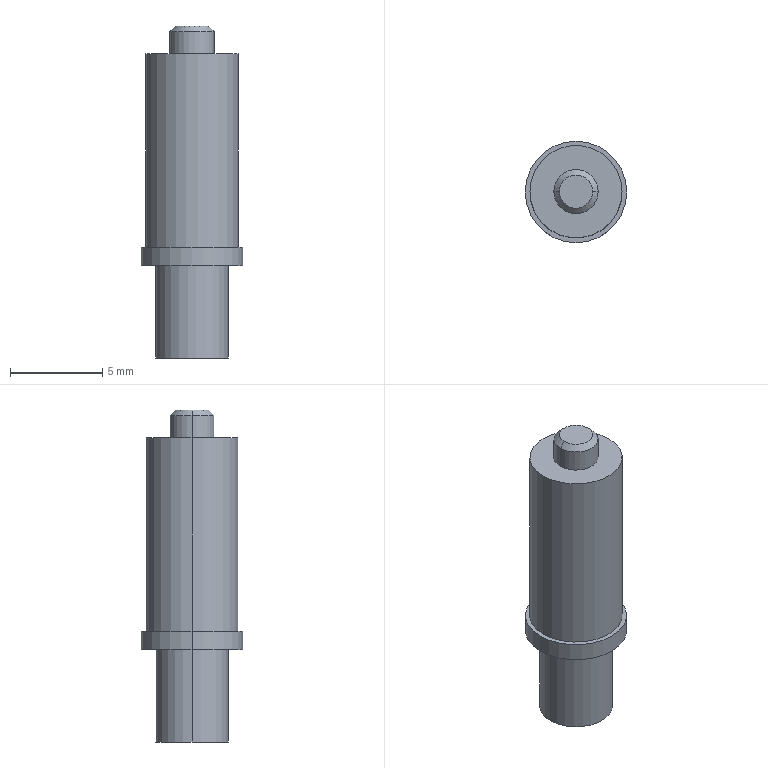Part | STEP file | 1 solid | 21 faces | box 5.5 x 5.5 x 18 mm | volume 266.671 mm3 | cylinder 10 | cone 6 | plane 5 | commonest cylinder face diameters 2.4 x2 2.5 x2 3.95 x2 5 x2 5.5 x2
STEP:
#1=CARTESIAN_POINT('',(0.,0.,0.));
#2=DIRECTION('',(0.,0.,1.));
#3=DIRECTION('',(1.,0.,0.));
#4=AXIS2_PLACEMENT_3D('',#1,#2,#3);
#5=CARTESIAN_POINT('',(-1.25,0.,0.275));
#6=VERTEX_POINT('',#5);
#7=CARTESIAN_POINT('',(-1.525,0.,0.));
#8=VERTEX_POINT('',#7);
#9=CARTESIAN_POINT('',(-1.525,0.,0.));
#10=DIRECTION('',(-0.7071,0.,-0.7071));
#11=VECTOR('',#10,1.);
#12=LINE('',#9,#11);
#13=CARTESIAN_POINT('',(0.,0.,0.));
#14=DIRECTION('',(0.,0.,-1.));
#15=DIRECTION('',(-1.,0.,0.));
#16=AXIS2_PLACEMENT_3D('',#13,#14,#15);
#17=CONICAL_SURFACE('',#16,1.525,0.7854);
#18=CARTESIAN_POINT('',(6.283,0.));
#19=DIRECTION('',(0.,1.));
#20=VECTOR('',#19,1.);
#21=LINE('',#18,#20);
#22=(GEOMETRIC_REPRESENTATION_CONTEXT(2)PARAMETRIC_REPRESENTATION_CONTEXT()REPRESENTATION_CONTEXT('',''));
#23=DEFINITIONAL_REPRESENTATION('',(#21),#22);
#24=PCURVE('',#17,#23);
#25=CARTESIAN_POINT('',(0.,0.,0.));
#26=DIRECTION('',(0.,0.,-1.));
#27=DIRECTION('',(-1.,0.,0.));
#28=AXIS2_PLACEMENT_3D('',#25,#26,#27);
#29=CONICAL_SURFACE('',#28,1.525,0.7854);
#30=CARTESIAN_POINT('',(0.,0.));
#31=DIRECTION('',(0.,1.));
#32=VECTOR('',#31,1.);
#33=LINE('',#30,#32);
#34=(GEOMETRIC_REPRESENTATION_CONTEXT(2)PARAMETRIC_REPRESENTATION_CONTEXT()REPRESENTATION_CONTEXT('',''));
#35=DEFINITIONAL_REPRESENTATION('',(#33),#34);
#36=PCURVE('',#29,#35);
#37=SURFACE_CURVE('',#12,(#24,#36),.PCURVE_S1.);
#38=EDGE_CURVE('',#6,#8,#37,.T.);
#39=ORIENTED_EDGE('',*,*,#38,.T.);
#40=CARTESIAN_POINT('',(1.525,0.,0.));
#41=VERTEX_POINT('',#40);
#42=CARTESIAN_POINT('',(0.,0.,0.));
#43=DIRECTION('',(0.,0.,-1.));
#44=DIRECTION('',(-1.,0.,0.));
#45=AXIS2_PLACEMENT_3D('',#42,#43,#44);
#46=CIRCLE('',#45,1.525);
#47=CARTESIAN_POINT('',(0.,0.));
#48=DIRECTION('',(1.,0.));
#49=VECTOR('',#48,1.);
#50=LINE('',#47,#49);
#51=(GEOMETRIC_REPRESENTATION_CONTEXT(2)PARAMETRIC_REPRESENTATION_CONTEXT()REPRESENTATION_CONTEXT('',''));
#52=DEFINITIONAL_REPRESENTATION('',(#50),#51);
#53=PCURVE('',#17,#52);
#54=CARTESIAN_POINT('',(0.,0.,0.));
#55=DIRECTION('',(0.,0.,-1.));
#56=DIRECTION('',(-1.,0.,0.));
#57=AXIS2_PLACEMENT_3D('',#54,#55,#56);
#58=PLANE('',#57);
#59=CARTESIAN_POINT('',(0.,0.));
#60=DIRECTION('',(1.,0.));
#61=AXIS2_PLACEMENT_2D('',#59,#60);
#62=CIRCLE('',#61,1.525);
#63=(GEOMETRIC_REPRESENTATION_CONTEXT(2)PARAMETRIC_REPRESENTATION_CONTEXT()REPRESENTATION_CONTEXT('',''));
#64=DEFINITIONAL_REPRESENTATION('',(#62),#63);
#65=PCURVE('',#58,#64);
#66=SURFACE_CURVE('',#46,(#53,#65),.PCURVE_S1.);
#67=EDGE_CURVE('',#41,#8,#66,.T.);
#68=ORIENTED_EDGE('',*,*,#67,.F.);
#69=CARTESIAN_POINT('',(1.25,0.,0.275));
#70=VERTEX_POINT('',#69);
#71=CARTESIAN_POINT('',(1.525,0.,0.));
#72=DIRECTION('',(0.7071,0.,-0.7071));
#73=VECTOR('',#72,1.);
#74=LINE('',#71,#73);
#75=CARTESIAN_POINT('',(3.142,0.));
#76=DIRECTION('',(0.,1.));
#77=VECTOR('',#76,1.);
#78=LINE('',#75,#77);
#79=(GEOMETRIC_REPRESENTATION_CONTEXT(2)PARAMETRIC_REPRESENTATION_CONTEXT()REPRESENTATION_CONTEXT('',''));
#80=DEFINITIONAL_REPRESENTATION('',(#78),#79);
#81=PCURVE('',#17,#80);
#82=CARTESIAN_POINT('',(3.142,0.));
#83=DIRECTION('',(0.,1.));
#84=VECTOR('',#83,1.);
#85=LINE('',#82,#84);
#86=(GEOMETRIC_REPRESENTATION_CONTEXT(2)PARAMETRIC_REPRESENTATION_CONTEXT()REPRESENTATION_CONTEXT('',''));
#87=DEFINITIONAL_REPRESENTATION('',(#85),#86);
#88=PCURVE('',#29,#87);
#89=SURFACE_CURVE('',#74,(#81,#88),.PCURVE_S1.);
#90=EDGE_CURVE('',#70,#41,#89,.T.);
#91=ORIENTED_EDGE('',*,*,#90,.F.);
#92=CARTESIAN_POINT('',(0.,0.,0.275));
#93=DIRECTION('',(0.,0.,-1.));
#94=DIRECTION('',(-1.,0.,0.));
#95=AXIS2_PLACEMENT_3D('',#92,#93,#94);
#96=CIRCLE('',#95,1.25);
#97=CARTESIAN_POINT('',(0.,-0.275));
#98=DIRECTION('',(1.,0.));
#99=VECTOR('',#98,1.);
#100=LINE('',#97,#99);
#101=(GEOMETRIC_REPRESENTATION_CONTEXT(2)PARAMETRIC_REPRESENTATION_CONTEXT()REPRESENTATION_CONTEXT('',''));
#102=DEFINITIONAL_REPRESENTATION('',(#100),#101);
#103=PCURVE('',#17,#102);
#104=CARTESIAN_POINT('',(0.,0.,0.));
#105=DIRECTION('',(0.,0.,-1.));
#106=DIRECTION('',(-1.,0.,0.));
#107=AXIS2_PLACEMENT_3D('',#104,#105,#106);
#108=CYLINDRICAL_SURFACE('',#107,1.25);
#109=CARTESIAN_POINT('',(0.,-0.275));
#110=DIRECTION('',(1.,0.));
#111=VECTOR('',#110,1.);
#112=LINE('',#109,#111);
#113=(GEOMETRIC_REPRESENTATION_CONTEXT(2)PARAMETRIC_REPRESENTATION_CONTEXT()REPRESENTATION_CONTEXT('',''));
#114=DEFINITIONAL_REPRESENTATION('',(#112),#113);
#115=PCURVE('',#108,#114);
#116=SURFACE_CURVE('',#96,(#103,#115),.PCURVE_S1.);
#117=EDGE_CURVE('',#70,#6,#116,.T.);
#118=ORIENTED_EDGE('',*,*,#117,.T.);
#119=EDGE_LOOP('',(#39,#68,#91,#118));
#120=FACE_BOUND('',#119,.F.);
#121=ADVANCED_FACE('',(#120),#17,.F.);
#122=CARTESIAN_POINT('',(-1.25,0.,6.));
#123=VERTEX_POINT('',#122);
#124=CARTESIAN_POINT('',(-1.25,0.,0.));
#125=DIRECTION('',(0.,0.,-1.));
#126=VECTOR('',#125,1.);
#127=LINE('',#124,#126);
#128=CARTESIAN_POINT('',(6.283,0.));
#129=DIRECTION('',(0.,1.));
#130=VECTOR('',#129,1.);
#131=LINE('',#128,#130);
#132=(GEOMETRIC_REPRESENTATION_CONTEXT(2)PARAMETRIC_REPRESENTATION_CONTEXT()REPRESENTATION_CONTEXT('',''));
#133=DEFINITIONAL_REPRESENTATION('',(#131),#132);
#134=PCURVE('',#108,#133);
#135=CARTESIAN_POINT('',(0.,0.,0.));
#136=DIRECTION('',(0.,0.,-1.));
#137=DIRECTION('',(-1.,0.,0.));
#138=AXIS2_PLACEMENT_3D('',#135,#136,#137);
#139=CYLINDRICAL_SURFACE('',#138,1.25);
#140=CARTESIAN_POINT('',(0.,0.));
#141=DIRECTION('',(0.,1.));
#142=VECTOR('',#141,1.);
#143=LINE('',#140,#142);
#144=(GEOMETRIC_REPRESENTATION_CONTEXT(2)PARAMETRIC_REPRESENTATION_CONTEXT()REPRESENTATION_CONTEXT('',''));
#145=DEFINITIONAL_REPRESENTATION('',(#143),#144);
#146=PCURVE('',#139,#145);
#147=SURFACE_CURVE('',#127,(#134,#146),.PCURVE_S1.);
#148=EDGE_CURVE('',#123,#6,#147,.T.);
#149=ORIENTED_EDGE('',*,*,#148,.T.);
#150=ORIENTED_EDGE('',*,*,#117,.F.);
#151=CARTESIAN_POINT('',(1.25,0.,6.));
#152=VERTEX_POINT('',#151);
#153=CARTESIAN_POINT('',(1.25,0.,0.));
#154=DIRECTION('',(0.,0.,-1.));
#155=VECTOR('',#154,1.);
#156=LINE('',#153,#155);
#157=CARTESIAN_POINT('',(3.142,0.));
#158=DIRECTION('',(0.,1.));
#159=VECTOR('',#158,1.);
#160=LINE('',#157,#159);
#161=(GEOMETRIC_REPRESENTATION_CONTEXT(2)PARAMETRIC_REPRESENTATION_CONTEXT()REPRESENTATION_CONTEXT('',''));
#162=DEFINITIONAL_REPRESENTATION('',(#160),#161);
#163=PCURVE('',#108,#162);
#164=CARTESIAN_POINT('',(3.142,0.));
#165=DIRECTION('',(0.,1.));
#166=VECTOR('',#165,1.);
#167=LINE('',#164,#166);
#168=(GEOMETRIC_REPRESENTATION_CONTEXT(2)PARAMETRIC_REPRESENTATION_CONTEXT()REPRESENTATION_CONTEXT('',''));
#169=DEFINITIONAL_REPRESENTATION('',(#167),#168);
#170=PCURVE('',#139,#169);
#171=SURFACE_CURVE('',#156,(#163,#170),.PCURVE_S1.);
#172=EDGE_CURVE('',#152,#70,#171,.T.);
#173=ORIENTED_EDGE('',*,*,#172,.F.);
#174=CARTESIAN_POINT('',(0.,0.,6.));
#175=DIRECTION('',(0.,0.,-1.));
#176=DIRECTION('',(-1.,0.,0.));
#177=AXIS2_PLACEMENT_3D('',#174,#175,#176);
#178=CIRCLE('',#177,1.25);
#179=CARTESIAN_POINT('',(0.,-6.));
#180=DIRECTION('',(1.,0.));
#181=VECTOR('',#180,1.);
#182=LINE('',#179,#181);
#183=(GEOMETRIC_REPRESENTATION_CONTEXT(2)PARAMETRIC_REPRESENTATION_CONTEXT()REPRESENTATION_CONTEXT('',''));
#184=DEFINITIONAL_REPRESENTATION('',(#182),#183);
#185=PCURVE('',#108,#184);
#186=CARTESIAN_POINT('',(0.,0.,6.));
#187=DIRECTION('',(0.,0.,-1.));
#188=DIRECTION('',(-1.,0.,0.));
#189=AXIS2_PLACEMENT_3D('',#186,#187,#188);
#190=CONICAL_SURFACE('',#189,1.25,1.03);
#191=CARTESIAN_POINT('',(0.,0.));
#192=DIRECTION('',(1.,0.));
#193=VECTOR('',#192,1.);
#194=LINE('',#191,#193);
#195=(GEOMETRIC_REPRESENTATION_CONTEXT(2)PARAMETRIC_REPRESENTATION_CONTEXT()REPRESENTATION_CONTEXT('',''));
#196=DEFINITIONAL_REPRESENTATION('',(#194),#195);
#197=PCURVE('',#190,#196);
#198=SURFACE_CURVE('',#178,(#185,#197),.PCURVE_S1.);
#199=EDGE_CURVE('',#152,#123,#198,.T.);
#200=ORIENTED_EDGE('',*,*,#199,.T.);
#201=EDGE_LOOP('',(#149,#150,#173,#200));
#202=FACE_BOUND('',#201,.F.);
#203=ADVANCED_FACE('',(#202),#108,.F.);
#204=ORIENTED_EDGE('',*,*,#199,.F.);
#205=CARTESIAN_POINT('',(0.,0.,6.751));
#206=VERTEX_POINT('',#205);
#207=CARTESIAN_POINT('',(1.25,0.,6.));
#208=DIRECTION('',(0.8572,0.,-0.515));
#209=VECTOR('',#208,1.);
#210=LINE('',#207,#209);
#211=CARTESIAN_POINT('',(3.142,0.));
#212=DIRECTION('',(0.,1.));
#213=VECTOR('',#212,1.);
#214=LINE('',#211,#213);
#215=(GEOMETRIC_REPRESENTATION_CONTEXT(2)PARAMETRIC_REPRESENTATION_CONTEXT()REPRESENTATION_CONTEXT('',''));
#216=DEFINITIONAL_REPRESENTATION('',(#214),#215);
#217=PCURVE('',#190,#216);
#218=CARTESIAN_POINT('',(0.,0.,6.));
#219=DIRECTION('',(0.,0.,-1.));
#220=DIRECTION('',(-1.,0.,0.));
#221=AXIS2_PLACEMENT_3D('',#218,#219,#220);
#222=CONICAL_SURFACE('',#221,1.25,1.03);
#223=CARTESIAN_POINT('',(3.142,0.));
#224=DIRECTION('',(0.,1.));
#225=VECTOR('',#224,1.);
#226=LINE('',#223,#225);
#227=(GEOMETRIC_REPRESENTATION_CONTEXT(2)PARAMETRIC_REPRESENTATION_CONTEXT()REPRESENTATION_CONTEXT('',''));
#228=DEFINITIONAL_REPRESENTATION('',(#226),#227);
#229=PCURVE('',#222,#228);
#230=SURFACE_CURVE('',#210,(#217,#229),.PCURVE_S1.);
#231=EDGE_CURVE('',#206,#152,#230,.T.);
#232=ORIENTED_EDGE('',*,*,#231,.F.);
#233=CARTESIAN_POINT('',(-1.25,0.,6.));
#234=DIRECTION('',(-0.8572,0.,-0.515));
#235=VECTOR('',#234,1.);
#236=LINE('',#233,#235);
#237=CARTESIAN_POINT('',(6.283,0.));
#238=DIRECTION('',(0.,1.));
#239=VECTOR('',#238,1.);
#240=LINE('',#237,#239);
#241=(GEOMETRIC_REPRESENTATION_CONTEXT(2)PARAMETRIC_REPRESENTATION_CONTEXT()REPRESENTATION_CONTEXT('',''));
#242=DEFINITIONAL_REPRESENTATION('',(#240),#241);
#243=PCURVE('',#190,#242);
#244=CARTESIAN_POINT('',(0.,0.));
#245=DIRECTION('',(0.,1.));
#246=VECTOR('',#245,1.);
#247=LINE('',#244,#246);
#248=(GEOMETRIC_REPRESENTATION_CONTEXT(2)PARAMETRIC_REPRESENTATION_CONTEXT()REPRESENTATION_CONTEXT('',''));
#249=DEFINITIONAL_REPRESENTATION('',(#247),#248);
#250=PCURVE('',#222,#249);
#251=SURFACE_CURVE('',#236,(#243,#250),.PCURVE_S1.);
#252=EDGE_CURVE('',#206,#123,#251,.T.);
#253=ORIENTED_EDGE('',*,*,#252,.T.);
#254=EDGE_LOOP('',(#204,#232,#253));
#255=FACE_BOUND('',#254,.F.);
#256=ADVANCED_FACE('',(#255),#190,.F.);
#257=CARTESIAN_POINT('',(0.9,0.,18.));
#258=VERTEX_POINT('',#257);
#259=CARTESIAN_POINT('',(-0.9,0.,18.));
#260=VERTEX_POINT('',#259);
#261=CARTESIAN_POINT('',(0.,0.,18.));
#262=DIRECTION('',(0.,0.,1.));
#263=DIRECTION('',(1.,0.,0.));
#264=AXIS2_PLACEMENT_3D('',#261,#262,#263);
#265=CIRCLE('',#264,0.9);
#266=CARTESIAN_POINT('',(0.,0.,18.));
#267=DIRECTION('',(0.,0.,-1.));
#268=DIRECTION('',(-1.,0.,0.));
#269=AXIS2_PLACEMENT_3D('',#266,#267,#268);
#270=CONICAL_SURFACE('',#269,0.9,0.7854);
#271=CARTESIAN_POINT('',(3.142,0.));
#272=DIRECTION('',(-1.,0.));
#273=VECTOR('',#272,1.);
#274=LINE('',#271,#273);
#275=(GEOMETRIC_REPRESENTATION_CONTEXT(2)PARAMETRIC_REPRESENTATION_CONTEXT()REPRESENTATION_CONTEXT('',''));
#276=DEFINITIONAL_REPRESENTATION('',(#274),#275);
#277=PCURVE('',#270,#276);
#278=CARTESIAN_POINT('',(0.9,0.,18.));
#279=DIRECTION('',(0.,0.,1.));
#280=DIRECTION('',(1.,0.,0.));
#281=AXIS2_PLACEMENT_3D('',#278,#279,#280);
#282=PLANE('',#281);
#283=CARTESIAN_POINT('',(-0.9,0.));
#284=DIRECTION('',(1.,0.));
#285=AXIS2_PLACEMENT_2D('',#283,#284);
#286=CIRCLE('',#285,0.9);
#287=(GEOMETRIC_REPRESENTATION_CONTEXT(2)PARAMETRIC_REPRESENTATION_CONTEXT()REPRESENTATION_CONTEXT('',''));
#288=DEFINITIONAL_REPRESENTATION('',(#286),#287);
#289=PCURVE('',#282,#288);
#290=SURFACE_CURVE('',#265,(#277,#289),.PCURVE_S1.);
#291=EDGE_CURVE('',#258,#260,#290,.T.);
#292=ORIENTED_EDGE('',*,*,#291,.F.);
#293=CARTESIAN_POINT('',(1.2,0.,17.7));
#294=VERTEX_POINT('',#293);
#295=CARTESIAN_POINT('',(0.9,0.,18.));
#296=DIRECTION('',(0.7071,0.,-0.7071));
#297=VECTOR('',#296,1.);
#298=LINE('',#295,#297);
#299=CARTESIAN_POINT('',(3.142,0.));
#300=DIRECTION('',(0.,1.));
#301=VECTOR('',#300,1.);
#302=LINE('',#299,#301);
#303=(GEOMETRIC_REPRESENTATION_CONTEXT(2)PARAMETRIC_REPRESENTATION_CONTEXT()REPRESENTATION_CONTEXT('',''));
#304=DEFINITIONAL_REPRESENTATION('',(#302),#303);
#305=PCURVE('',#270,#304);
#306=CARTESIAN_POINT('',(0.,0.,18.));
#307=DIRECTION('',(0.,0.,-1.));
#308=DIRECTION('',(-1.,0.,0.));
#309=AXIS2_PLACEMENT_3D('',#306,#307,#308);
#310=CONICAL_SURFACE('',#309,0.9,0.7854);
#311=CARTESIAN_POINT('',(3.142,0.));
#312=DIRECTION('',(0.,1.));
#313=VECTOR('',#312,1.);
#314=LINE('',#311,#313);
#315=(GEOMETRIC_REPRESENTATION_CONTEXT(2)PARAMETRIC_REPRESENTATION_CONTEXT()REPRESENTATION_CONTEXT('',''));
#316=DEFINITIONAL_REPRESENTATION('',(#314),#315);
#317=PCURVE('',#310,#316);
#318=SURFACE_CURVE('',#298,(#305,#317),.PCURVE_S1.);
#319=EDGE_CURVE('',#258,#294,#318,.T.);
#320=ORIENTED_EDGE('',*,*,#319,.T.);
#321=CARTESIAN_POINT('',(-1.2,0.,17.7));
#322=VERTEX_POINT('',#321);
#323=CARTESIAN_POINT('',(0.,0.,17.7));
#324=DIRECTION('',(0.,0.,1.));
#325=DIRECTION('',(1.,0.,0.));
#326=AXIS2_PLACEMENT_3D('',#323,#324,#325);
#327=CIRCLE('',#326,1.2);
#328=CARTESIAN_POINT('',(3.142,0.3));
#329=DIRECTION('',(-1.,0.));
#330=VECTOR('',#329,1.);
#331=LINE('',#328,#330);
#332=(GEOMETRIC_REPRESENTATION_CONTEXT(2)PARAMETRIC_REPRESENTATION_CONTEXT()REPRESENTATION_CONTEXT('',''));
#333=DEFINITIONAL_REPRESENTATION('',(#331),#332);
#334=PCURVE('',#270,#333);
#335=CARTESIAN_POINT('',(0.,0.,0.));
#336=DIRECTION('',(0.,0.,1.));
#337=DIRECTION('',(1.,0.,0.));
#338=AXIS2_PLACEMENT_3D('',#335,#336,#337);
#339=CYLINDRICAL_SURFACE('',#338,1.2);
#340=CARTESIAN_POINT('',(0.,17.7));
#341=DIRECTION('',(1.,0.));
#342=VECTOR('',#341,1.);
#343=LINE('',#340,#342);
#344=(GEOMETRIC_REPRESENTATION_CONTEXT(2)PARAMETRIC_REPRESENTATION_CONTEXT()REPRESENTATION_CONTEXT('',''));
#345=DEFINITIONAL_REPRESENTATION('',(#343),#344);
#346=PCURVE('',#339,#345);
#347=SURFACE_CURVE('',#327,(#334,#346),.PCURVE_S1.);
#348=EDGE_CURVE('',#294,#322,#347,.T.);
#349=ORIENTED_EDGE('',*,*,#348,.T.);
#350=CARTESIAN_POINT('',(-0.9,0.,18.));
#351=DIRECTION('',(-0.7071,0.,-0.7071));
#352=VECTOR('',#351,1.);
#353=LINE('',#350,#352);
#354=CARTESIAN_POINT('',(0.,0.));
#355=DIRECTION('',(0.,1.));
#356=VECTOR('',#355,1.);
#357=LINE('',#354,#356);
#358=(GEOMETRIC_REPRESENTATION_CONTEXT(2)PARAMETRIC_REPRESENTATION_CONTEXT()REPRESENTATION_CONTEXT('',''));
#359=DEFINITIONAL_REPRESENTATION('',(#357),#358);
#360=PCURVE('',#270,#359);
#361=CARTESIAN_POINT('',(6.283,0.));
#362=DIRECTION('',(0.,1.));
#363=VECTOR('',#362,1.);
#364=LINE('',#361,#363);
#365=(GEOMETRIC_REPRESENTATION_CONTEXT(2)PARAMETRIC_REPRESENTATION_CONTEXT()REPRESENTATION_CONTEXT('',''));
#366=DEFINITIONAL_REPRESENTATION('',(#364),#365);
#367=PCURVE('',#310,#366);
#368=SURFACE_CURVE('',#353,(#360,#367),.PCURVE_S1.);
#369=EDGE_CURVE('',#260,#322,#368,.T.);
#370=ORIENTED_EDGE('',*,*,#369,.F.);
#371=EDGE_LOOP('',(#292,#320,#349,#370));
#372=FACE_BOUND('',#371,.T.);
#373=ADVANCED_FACE('',(#372),#270,.T.);
#374=CARTESIAN_POINT('',(1.2,0.,16.5));
#375=VERTEX_POINT('',#374);
#376=CARTESIAN_POINT('',(-1.2,0.,16.5));
#377=VERTEX_POINT('',#376);
#378=CARTESIAN_POINT('',(0.,0.,16.5));
#379=DIRECTION('',(0.,0.,1.));
#380=DIRECTION('',(1.,0.,0.));
#381=AXIS2_PLACEMENT_3D('',#378,#379,#380);
#382=CIRCLE('',#381,1.2);
#383=CARTESIAN_POINT('',(0.,16.5));
#384=DIRECTION('',(1.,0.));
#385=VECTOR('',#384,1.);
#386=LINE('',#383,#385);
#387=(GEOMETRIC_REPRESENTATION_CONTEXT(2)PARAMETRIC_REPRESENTATION_CONTEXT()REPRESENTATION_CONTEXT('',''));
#388=DEFINITIONAL_REPRESENTATION('',(#386),#387);
#389=PCURVE('',#339,#388);
#390=CARTESIAN_POINT('',(2.5,0.,16.5));
#391=DIRECTION('',(0.,0.,1.));
#392=DIRECTION('',(1.,0.,0.));
#393=AXIS2_PLACEMENT_3D('',#390,#391,#392);
#394=PLANE('',#393);
#395=CARTESIAN_POINT('',(-2.5,0.));
#396=DIRECTION('',(1.,0.));
#397=AXIS2_PLACEMENT_2D('',#395,#396);
#398=CIRCLE('',#397,1.2);
#399=(GEOMETRIC_REPRESENTATION_CONTEXT(2)PARAMETRIC_REPRESENTATION_CONTEXT()REPRESENTATION_CONTEXT('',''));
#400=DEFINITIONAL_REPRESENTATION('',(#398),#399);
#401=PCURVE('',#394,#400);
#402=SURFACE_CURVE('',#382,(#389,#401),.PCURVE_S1.);
#403=EDGE_CURVE('',#375,#377,#402,.T.);
#404=ORIENTED_EDGE('',*,*,#403,.T.);
#405=CARTESIAN_POINT('',(-1.2,0.,0.));
#406=DIRECTION('',(0.,0.,1.));
#407=VECTOR('',#406,1.);
#408=LINE('',#405,#407);
#409=CARTESIAN_POINT('',(3.142,0.));
#410=DIRECTION('',(0.,1.));
#411=VECTOR('',#410,1.);
#412=LINE('',#409,#411);
#413=(GEOMETRIC_REPRESENTATION_CONTEXT(2)PARAMETRIC_REPRESENTATION_CONTEXT()REPRESENTATION_CONTEXT('',''));
#414=DEFINITIONAL_REPRESENTATION('',(#412),#413);
#415=PCURVE('',#339,#414);
#416=CARTESIAN_POINT('',(0.,0.,0.));
#417=DIRECTION('',(0.,0.,1.));
#418=DIRECTION('',(1.,0.,0.));
#419=AXIS2_PLACEMENT_3D('',#416,#417,#418);
#420=CYLINDRICAL_SURFACE('',#419,1.2);
#421=CARTESIAN_POINT('',(3.142,0.));
#422=DIRECTION('',(0.,1.));
#423=VECTOR('',#422,1.);
#424=LINE('',#421,#423);
#425=(GEOMETRIC_REPRESENTATION_CONTEXT(2)PARAMETRIC_REPRESENTATION_CONTEXT()REPRESENTATION_CONTEXT('',''));
#426=DEFINITIONAL_REPRESENTATION('',(#424),#425);
#427=PCURVE('',#420,#426);
#428=SURFACE_CURVE('',#408,(#415,#427),.PCURVE_S1.);
#429=EDGE_CURVE('',#377,#322,#428,.T.);
#430=ORIENTED_EDGE('',*,*,#429,.T.);
#431=ORIENTED_EDGE('',*,*,#348,.F.);
#432=CARTESIAN_POINT('',(1.2,0.,0.));
#433=DIRECTION('',(0.,0.,1.));
#434=VECTOR('',#433,1.);
#435=LINE('',#432,#434);
#436=CARTESIAN_POINT('',(0.,0.));
#437=DIRECTION('',(0.,1.));
#438=VECTOR('',#437,1.);
#439=LINE('',#436,#438);
#440=(GEOMETRIC_REPRESENTATION_CONTEXT(2)PARAMETRIC_REPRESENTATION_CONTEXT()REPRESENTATION_CONTEXT('',''));
#441=DEFINITIONAL_REPRESENTATION('',(#439),#440);
#442=PCURVE('',#339,#441);
#443=CARTESIAN_POINT('',(6.283,0.));
#444=DIRECTION('',(0.,1.));
#445=VECTOR('',#444,1.);
#446=LINE('',#443,#445);
#447=(GEOMETRIC_REPRESENTATION_CONTEXT(2)PARAMETRIC_REPRESENTATION_CONTEXT()REPRESENTATION_CONTEXT('',''));
#448=DEFINITIONAL_REPRESENTATION('',(#446),#447);
#449=PCURVE('',#420,#448);
#450=SURFACE_CURVE('',#435,(#442,#449),.PCURVE_S1.);
#451=EDGE_CURVE('',#375,#294,#450,.T.);
#452=ORIENTED_EDGE('',*,*,#451,.F.);
#453=EDGE_LOOP('',(#404,#430,#431,#452));
#454=FACE_BOUND('',#453,.T.);
#455=ADVANCED_FACE('',(#454),#339,.T.);
#456=CARTESIAN_POINT('',(2.5,0.,6.));
#457=VERTEX_POINT('',#456);
#458=CARTESIAN_POINT('',(-2.5,0.,6.));
#459=VERTEX_POINT('',#458);
#460=CARTESIAN_POINT('',(0.,0.,6.));
#461=DIRECTION('',(0.,0.,1.));
#462=DIRECTION('',(1.,0.,0.));
#463=AXIS2_PLACEMENT_3D('',#460,#461,#462);
#464=CIRCLE('',#463,2.5);
#465=CARTESIAN_POINT('',(0.,0.,0.));
#466=DIRECTION('',(0.,0.,1.));
#467=DIRECTION('',(1.,0.,0.));
#468=AXIS2_PLACEMENT_3D('',#465,#466,#467);
#469=CYLINDRICAL_SURFACE('',#468,2.5);
#470=CARTESIAN_POINT('',(0.,6.));
#471=DIRECTION('',(1.,0.));
#472=VECTOR('',#471,1.);
#473=LINE('',#470,#472);
#474=(GEOMETRIC_REPRESENTATION_CONTEXT(2)PARAMETRIC_REPRESENTATION_CONTEXT()REPRESENTATION_CONTEXT('',''));
#475=DEFINITIONAL_REPRESENTATION('',(#473),#474);
#476=PCURVE('',#469,#475);
#477=CARTESIAN_POINT('',(2.75,0.,6.));
#478=DIRECTION('',(0.,0.,1.));
#479=DIRECTION('',(1.,0.,0.));
#480=AXIS2_PLACEMENT_3D('',#477,#478,#479);
#481=PLANE('',#480);
#482=CARTESIAN_POINT('',(-2.75,0.));
#483=DIRECTION('',(1.,0.));
#484=AXIS2_PLACEMENT_2D('',#482,#483);
#485=CIRCLE('',#484,2.5);
#486=(GEOMETRIC_REPRESENTATION_CONTEXT(2)PARAMETRIC_REPRESENTATION_CONTEXT()REPRESENTATION_CONTEXT('',''));
#487=DEFINITIONAL_REPRESENTATION('',(#485),#486);
#488=PCURVE('',#481,#487);
#489=SURFACE_CURVE('',#464,(#476,#488),.PCURVE_S1.);
#490=EDGE_CURVE('',#457,#459,#489,.T.);
#491=ORIENTED_EDGE('',*,*,#490,.T.);
#492=CARTESIAN_POINT('',(-2.5,0.,16.5));
#493=VERTEX_POINT('',#492);
#494=CARTESIAN_POINT('',(-2.5,0.,0.));
#495=DIRECTION('',(0.,0.,1.));
#496=VECTOR('',#495,1.);
#497=LINE('',#494,#496);
#498=CARTESIAN_POINT('',(3.142,0.));
#499=DIRECTION('',(0.,1.));
#500=VECTOR('',#499,1.);
#501=LINE('',#498,#500);
#502=(GEOMETRIC_REPRESENTATION_CONTEXT(2)PARAMETRIC_REPRESENTATION_CONTEXT()REPRESENTATION_CONTEXT('',''));
#503=DEFINITIONAL_REPRESENTATION('',(#501),#502);
#504=PCURVE('',#469,#503);
#505=CARTESIAN_POINT('',(0.,0.,0.));
#506=DIRECTION('',(0.,0.,1.));
#507=DIRECTION('',(1.,0.,0.));
#508=AXIS2_PLACEMENT_3D('',#505,#506,#507);
#509=CYLINDRICAL_SURFACE('',#508,2.5);
#510=CARTESIAN_POINT('',(3.142,0.));
#511=DIRECTION('',(0.,1.));
#512=VECTOR('',#511,1.);
#513=LINE('',#510,#512);
#514=(GEOMETRIC_REPRESENTATION_CONTEXT(2)PARAMETRIC_REPRESENTATION_CONTEXT()REPRESENTATION_CONTEXT('',''));
#515=DEFINITIONAL_REPRESENTATION('',(#513),#514);
#516=PCURVE('',#509,#515);
#517=SURFACE_CURVE('',#497,(#504,#516),.PCURVE_S1.);
#518=EDGE_CURVE('',#459,#493,#517,.T.);
#519=ORIENTED_EDGE('',*,*,#518,.T.);
#520=CARTESIAN_POINT('',(2.5,0.,16.5));
#521=VERTEX_POINT('',#520);
#522=CARTESIAN_POINT('',(0.,0.,16.5));
#523=DIRECTION('',(0.,0.,1.));
#524=DIRECTION('',(1.,0.,0.));
#525=AXIS2_PLACEMENT_3D('',#522,#523,#524);
#526=CIRCLE('',#525,2.5);
#527=CARTESIAN_POINT('',(0.,16.5));
#528=DIRECTION('',(1.,0.));
#529=VECTOR('',#528,1.);
#530=LINE('',#527,#529);
#531=(GEOMETRIC_REPRESENTATION_CONTEXT(2)PARAMETRIC_REPRESENTATION_CONTEXT()REPRESENTATION_CONTEXT('',''));
#532=DEFINITIONAL_REPRESENTATION('',(#530),#531);
#533=PCURVE('',#469,#532);
#534=CARTESIAN_POINT('',(-2.5,0.));
#535=DIRECTION('',(1.,0.));
#536=AXIS2_PLACEMENT_2D('',#534,#535);
#537=CIRCLE('',#536,2.5);
#538=(GEOMETRIC_REPRESENTATION_CONTEXT(2)PARAMETRIC_REPRESENTATION_CONTEXT()REPRESENTATION_CONTEXT('',''));
#539=DEFINITIONAL_REPRESENTATION('',(#537),#538);
#540=PCURVE('',#394,#539);
#541=SURFACE_CURVE('',#526,(#533,#540),.PCURVE_S1.);
#542=EDGE_CURVE('',#521,#493,#541,.T.);
#543=ORIENTED_EDGE('',*,*,#542,.F.);
#544=CARTESIAN_POINT('',(2.5,0.,0.));
#545=DIRECTION('',(0.,0.,1.));
#546=VECTOR('',#545,1.);
#547=LINE('',#544,#546);
#548=CARTESIAN_POINT('',(0.,0.));
#549=DIRECTION('',(0.,1.));
#550=VECTOR('',#549,1.);
#551=LINE('',#548,#550);
#552=(GEOMETRIC_REPRESENTATION_CONTEXT(2)PARAMETRIC_REPRESENTATION_CONTEXT()REPRESENTATION_CONTEXT('',''));
#553=DEFINITIONAL_REPRESENTATION('',(#551),#552);
#554=PCURVE('',#469,#553);
#555=CARTESIAN_POINT('',(6.283,0.));
#556=DIRECTION('',(0.,1.));
#557=VECTOR('',#556,1.);
#558=LINE('',#555,#557);
#559=(GEOMETRIC_REPRESENTATION_CONTEXT(2)PARAMETRIC_REPRESENTATION_CONTEXT()REPRESENTATION_CONTEXT('',''));
#560=DEFINITIONAL_REPRESENTATION('',(#558),#559);
#561=PCURVE('',#509,#560);
#562=SURFACE_CURVE('',#547,(#554,#561),.PCURVE_S1.);
#563=EDGE_CURVE('',#457,#521,#562,.T.);
#564=ORIENTED_EDGE('',*,*,#563,.F.);
#565=EDGE_LOOP('',(#491,#519,#543,#564));
#566=FACE_BOUND('',#565,.T.);
#567=ADVANCED_FACE('',(#566),#469,.T.);
#568=CARTESIAN_POINT('',(2.75,0.,5.));
#569=VERTEX_POINT('',#568);
#570=CARTESIAN_POINT('',(-2.75,0.,5.));
#571=VERTEX_POINT('',#570);
#572=CARTESIAN_POINT('',(0.,0.,5.));
#573=DIRECTION('',(0.,0.,1.));
#574=DIRECTION('',(1.,0.,0.));
#575=AXIS2_PLACEMENT_3D('',#572,#573,#574);
#576=CIRCLE('',#575,2.75);
#577=CARTESIAN_POINT('',(0.,0.,0.));
#578=DIRECTION('',(0.,0.,1.));
#579=DIRECTION('',(1.,0.,0.));
#580=AXIS2_PLACEMENT_3D('',#577,#578,#579);
#581=CYLINDRICAL_SURFACE('',#580,2.75);
#582=CARTESIAN_POINT('',(0.,5.));
#583=DIRECTION('',(1.,0.));
#584=VECTOR('',#583,1.);
#585=LINE('',#582,#584);
#586=(GEOMETRIC_REPRESENTATION_CONTEXT(2)PARAMETRIC_REPRESENTATION_CONTEXT()REPRESENTATION_CONTEXT('',''));
#587=DEFINITIONAL_REPRESENTATION('',(#585),#586);
#588=PCURVE('',#581,#587);
#589=CARTESIAN_POINT('',(1.975,0.,5.));
#590=DIRECTION('',(0.,0.,-1.));
#591=DIRECTION('',(-1.,0.,0.));
#592=AXIS2_PLACEMENT_3D('',#589,#590,#591);
#593=PLANE('',#592);
#594=CARTESIAN_POINT('',(-0.775,0.));
#595=CARTESIAN_POINT('',(-0.775,4.763));
#596=CARTESIAN_POINT('',(3.35,2.382));
#597=CARTESIAN_POINT('',(7.475,0.));
#598=CARTESIAN_POINT('',(3.35,-2.382));
#599=CARTESIAN_POINT('',(-0.775,-4.763));
#600=CARTESIAN_POINT('',(-0.775,0.));
#601=(BOUNDED_CURVE()B_SPLINE_CURVE(2,(#594,#595,#596,#597,#598,#599,#600),.UNSPECIFIED.,.T.,.F.)B_SPLINE_CURVE_WITH_KNOTS((1,2,2,2,2,1),(-2.094,0.,2.094,4.189,6.283,8.378),.UNSPECIFIED.)CURVE()GEOMETRIC_REPRESENTATION_ITEM()RATIONAL_B_SPLINE_CURVE((1.,0.5,1.,0.5,1.,0.5,1.))REPRESENTATION_ITEM(''));
#602=(GEOMETRIC_REPRESENTATION_CONTEXT(2)PARAMETRIC_REPRESENTATION_CONTEXT()REPRESENTATION_CONTEXT('',''));
#603=DEFINITIONAL_REPRESENTATION('',(#601),#602);
#604=PCURVE('',#593,#603);
#605=SURFACE_CURVE('',#576,(#588,#604),.PCURVE_S1.);
#606=EDGE_CURVE('',#569,#571,#605,.T.);
#607=ORIENTED_EDGE('',*,*,#606,.T.);
#608=CARTESIAN_POINT('',(-2.75,0.,6.));
#609=VERTEX_POINT('',#608);
#610=CARTESIAN_POINT('',(-2.75,0.,0.));
#611=DIRECTION('',(0.,0.,1.));
#612=VECTOR('',#611,1.);
#613=LINE('',#610,#612);
#614=CARTESIAN_POINT('',(3.142,0.));
#615=DIRECTION('',(0.,1.));
#616=VECTOR('',#615,1.);
#617=LINE('',#614,#616);
#618=(GEOMETRIC_REPRESENTATION_CONTEXT(2)PARAMETRIC_REPRESENTATION_CONTEXT()REPRESENTATION_CONTEXT('',''));
#619=DEFINITIONAL_REPRESENTATION('',(#617),#618);
#620=PCURVE('',#581,#619);
#621=CARTESIAN_POINT('',(0.,0.,0.));
#622=DIRECTION('',(0.,0.,1.));
#623=DIRECTION('',(1.,0.,0.));
#624=AXIS2_PLACEMENT_3D('',#621,#622,#623);
#625=CYLINDRICAL_SURFACE('',#624,2.75);
#626=CARTESIAN_POINT('',(3.142,0.));
#627=DIRECTION('',(0.,1.));
#628=VECTOR('',#627,1.);
#629=LINE('',#626,#628);
#630=(GEOMETRIC_REPRESENTATION_CONTEXT(2)PARAMETRIC_REPRESENTATION_CONTEXT()REPRESENTATION_CONTEXT('',''));
#631=DEFINITIONAL_REPRESENTATION('',(#629),#630);
#632=PCURVE('',#625,#631);
#633=SURFACE_CURVE('',#613,(#620,#632),.PCURVE_S1.);
#634=EDGE_CURVE('',#571,#609,#633,.T.);
#635=ORIENTED_EDGE('',*,*,#634,.T.);
#636=CARTESIAN_POINT('',(2.75,0.,6.));
#637=VERTEX_POINT('',#636);
#638=CARTESIAN_POINT('',(0.,0.,6.));
#639=DIRECTION('',(0.,0.,1.));
#640=DIRECTION('',(1.,0.,0.));
#641=AXIS2_PLACEMENT_3D('',#638,#639,#640);
#642=CIRCLE('',#641,2.75);
#643=CARTESIAN_POINT('',(0.,6.));
#644=DIRECTION('',(1.,0.));
#645=VECTOR('',#644,1.);
#646=LINE('',#643,#645);
#647=(GEOMETRIC_REPRESENTATION_CONTEXT(2)PARAMETRIC_REPRESENTATION_CONTEXT()REPRESENTATION_CONTEXT('',''));
#648=DEFINITIONAL_REPRESENTATION('',(#646),#647);
#649=PCURVE('',#581,#648);
#650=CARTESIAN_POINT('',(-2.75,0.));
#651=DIRECTION('',(1.,0.));
#652=AXIS2_PLACEMENT_2D('',#650,#651);
#653=CIRCLE('',#652,2.75);
#654=(GEOMETRIC_REPRESENTATION_CONTEXT(2)PARAMETRIC_REPRESENTATION_CONTEXT()REPRESENTATION_CONTEXT('',''));
#655=DEFINITIONAL_REPRESENTATION('',(#653),#654);
#656=PCURVE('',#481,#655);
#657=SURFACE_CURVE('',#642,(#649,#656),.PCURVE_S1.);
#658=EDGE_CURVE('',#637,#609,#657,.T.);
#659=ORIENTED_EDGE('',*,*,#658,.F.);
#660=CARTESIAN_POINT('',(2.75,0.,0.));
#661=DIRECTION('',(0.,0.,1.));
#662=VECTOR('',#661,1.);
#663=LINE('',#660,#662);
#664=CARTESIAN_POINT('',(0.,0.));
#665=DIRECTION('',(0.,1.));
#666=VECTOR('',#665,1.);
#667=LINE('',#664,#666);
#668=(GEOMETRIC_REPRESENTATION_CONTEXT(2)PARAMETRIC_REPRESENTATION_CONTEXT()REPRESENTATION_CONTEXT('',''));
#669=DEFINITIONAL_REPRESENTATION('',(#667),#668);
#670=PCURVE('',#581,#669);
#671=CARTESIAN_POINT('',(6.283,0.));
#672=DIRECTION('',(0.,1.));
#673=VECTOR('',#672,1.);
#674=LINE('',#671,#673);
#675=(GEOMETRIC_REPRESENTATION_CONTEXT(2)PARAMETRIC_REPRESENTATION_CONTEXT()REPRESENTATION_CONTEXT('',''));
#676=DEFINITIONAL_REPRESENTATION('',(#674),#675);
#677=PCURVE('',#625,#676);
#678=SURFACE_CURVE('',#663,(#670,#677),.PCURVE_S1.);
#679=EDGE_CURVE('',#569,#637,#678,.T.);
#680=ORIENTED_EDGE('',*,*,#679,.F.);
#681=EDGE_LOOP('',(#607,#635,#659,#680));
#682=FACE_BOUND('',#681,.T.);
#683=ADVANCED_FACE('',(#682),#581,.T.);
#684=CARTESIAN_POINT('',(1.975,0.,0.));
#685=VERTEX_POINT('',#684);
#686=CARTESIAN_POINT('',(-1.975,0.,0.));
#687=VERTEX_POINT('',#686);
#688=CARTESIAN_POINT('',(0.,0.,0.));
#689=DIRECTION('',(0.,0.,1.));
#690=DIRECTION('',(1.,0.,0.));
#691=AXIS2_PLACEMENT_3D('',#688,#689,#690);
#692=CIRCLE('',#691,1.975);
#693=CARTESIAN_POINT('',(0.,0.,0.));
#694=DIRECTION('',(0.,0.,1.));
#695=DIRECTION('',(1.,0.,0.));
#696=AXIS2_PLACEMENT_3D('',#693,#694,#695);
#697=CYLINDRICAL_SURFACE('',#696,1.975);
#698=CARTESIAN_POINT('',(0.,0.));
#699=DIRECTION('',(1.,0.));
#700=VECTOR('',#699,1.);
#701=LINE('',#698,#700);
#702=(GEOMETRIC_REPRESENTATION_CONTEXT(2)PARAMETRIC_REPRESENTATION_CONTEXT()REPRESENTATION_CONTEXT('',''));
#703=DEFINITIONAL_REPRESENTATION('',(#701),#702);
#704=PCURVE('',#697,#703);
#705=CARTESIAN_POINT('',(-1.975,0.));
#706=CARTESIAN_POINT('',(-1.975,3.421));
#707=CARTESIAN_POINT('',(0.9875,1.71));
#708=CARTESIAN_POINT('',(3.95,0.));
#709=CARTESIAN_POINT('',(0.9875,-1.71));
#710=CARTESIAN_POINT('',(-1.975,-3.421));
#711=CARTESIAN_POINT('',(-1.975,0.));
#712=(BOUNDED_CURVE()B_SPLINE_CURVE(2,(#705,#706,#707,#708,#709,#710,#711),.UNSPECIFIED.,.T.,.F.)B_SPLINE_CURVE_WITH_KNOTS((1,2,2,2,2,1),(-2.094,0.,2.094,4.189,6.283,8.378),.UNSPECIFIED.)CURVE()GEOMETRIC_REPRESENTATION_ITEM()RATIONAL_B_SPLINE_CURVE((1.,0.5,1.,0.5,1.,0.5,1.))REPRESENTATION_ITEM(''));
#713=(GEOMETRIC_REPRESENTATION_CONTEXT(2)PARAMETRIC_REPRESENTATION_CONTEXT()REPRESENTATION_CONTEXT('',''));
#714=DEFINITIONAL_REPRESENTATION('',(#712),#713);
#715=PCURVE('',#58,#714);
#716=SURFACE_CURVE('',#692,(#704,#715),.PCURVE_S1.);
#717=EDGE_CURVE('',#685,#687,#716,.T.);
#718=ORIENTED_EDGE('',*,*,#717,.T.);
#719=CARTESIAN_POINT('',(-1.975,0.,5.));
#720=VERTEX_POINT('',#719);
#721=CARTESIAN_POINT('',(-1.975,0.,0.));
#722=DIRECTION('',(0.,0.,1.));
#723=VECTOR('',#722,1.);
#724=LINE('',#721,#723);
#725=CARTESIAN_POINT('',(3.142,0.));
#726=DIRECTION('',(0.,1.));
#727=VECTOR('',#726,1.);
#728=LINE('',#725,#727);
#729=(GEOMETRIC_REPRESENTATION_CONTEXT(2)PARAMETRIC_REPRESENTATION_CONTEXT()REPRESENTATION_CONTEXT('',''));
#730=DEFINITIONAL_REPRESENTATION('',(#728),#729);
#731=PCURVE('',#697,#730);
#732=CARTESIAN_POINT('',(0.,0.,0.));
#733=DIRECTION('',(0.,0.,1.));
#734=DIRECTION('',(1.,0.,0.));
#735=AXIS2_PLACEMENT_3D('',#732,#733,#734);
#736=CYLINDRICAL_SURFACE('',#735,1.975);
#737=CARTESIAN_POINT('',(3.142,0.));
#738=DIRECTION('',(0.,1.));
#739=VECTOR('',#738,1.);
#740=LINE('',#737,#739);
#741=(GEOMETRIC_REPRESENTATION_CONTEXT(2)PARAMETRIC_REPRESENTATION_CONTEXT()REPRESENTATION_CONTEXT('',''));
#742=DEFINITIONAL_REPRESENTATION('',(#740),#741);
#743=PCURVE('',#736,#742);
#744=SURFACE_CURVE('',#724,(#731,#743),.PCURVE_S1.);
#745=EDGE_CURVE('',#687,#720,#744,.T.);
#746=ORIENTED_EDGE('',*,*,#745,.T.);
#747=CARTESIAN_POINT('',(1.975,0.,5.));
#748=VERTEX_POINT('',#747);
#749=CARTESIAN_POINT('',(0.,0.,5.));
#750=DIRECTION('',(0.,0.,1.));
#751=DIRECTION('',(1.,0.,0.));
#752=AXIS2_PLACEMENT_3D('',#749,#750,#751);
#753=CIRCLE('',#752,1.975);
#754=CARTESIAN_POINT('',(0.,5.));
#755=DIRECTION('',(1.,0.));
#756=VECTOR('',#755,1.);
#757=LINE('',#754,#756);
#758=(GEOMETRIC_REPRESENTATION_CONTEXT(2)PARAMETRIC_REPRESENTATION_CONTEXT()REPRESENTATION_CONTEXT('',''));
#759=DEFINITIONAL_REPRESENTATION('',(#757),#758);
#760=PCURVE('',#697,#759);
#761=CARTESIAN_POINT('',(0.,0.));
#762=CARTESIAN_POINT('',(0.,3.421));
#763=CARTESIAN_POINT('',(2.962,1.71));
#764=CARTESIAN_POINT('',(5.925,0.));
#765=CARTESIAN_POINT('',(2.962,-1.71));
#766=CARTESIAN_POINT('',(0.,-3.421));
#767=CARTESIAN_POINT('',(0.,0.));
#768=(BOUNDED_CURVE()B_SPLINE_CURVE(2,(#761,#762,#763,#764,#765,#766,#767),.UNSPECIFIED.,.T.,.F.)B_SPLINE_CURVE_WITH_KNOTS((1,2,2,2,2,1),(-2.094,0.,2.094,4.189,6.283,8.378),.UNSPECIFIED.)CURVE()GEOMETRIC_REPRESENTATION_ITEM()RATIONAL_B_SPLINE_CURVE((1.,0.5,1.,0.5,1.,0.5,1.))REPRESENTATION_ITEM(''));
#769=(GEOMETRIC_REPRESENTATION_CONTEXT(2)PARAMETRIC_REPRESENTATION_CONTEXT()REPRESENTATION_CONTEXT('',''));
#770=DEFINITIONAL_REPRESENTATION('',(#768),#769);
#771=PCURVE('',#593,#770);
#772=SURFACE_CURVE('',#753,(#760,#771),.PCURVE_S1.);
#773=EDGE_CURVE('',#748,#720,#772,.T.);
#774=ORIENTED_EDGE('',*,*,#773,.F.);
#775=CARTESIAN_POINT('',(1.975,0.,0.));
#776=DIRECTION('',(0.,0.,1.));
#777=VECTOR('',#776,1.);
#778=LINE('',#775,#777);
#779=CARTESIAN_POINT('',(0.,0.));
#780=DIRECTION('',(0.,1.));
#781=VECTOR('',#780,1.);
#782=LINE('',#779,#781);
#783=(GEOMETRIC_REPRESENTATION_CONTEXT(2)PARAMETRIC_REPRESENTATION_CONTEXT()REPRESENTATION_CONTEXT('',''));
#784=DEFINITIONAL_REPRESENTATION('',(#782),#783);
#785=PCURVE('',#697,#784);
#786=CARTESIAN_POINT('',(6.283,0.));
#787=DIRECTION('',(0.,1.));
#788=VECTOR('',#787,1.);
#789=LINE('',#786,#788);
#790=(GEOMETRIC_REPRESENTATION_CONTEXT(2)PARAMETRIC_REPRESENTATION_CONTEXT()REPRESENTATION_CONTEXT('',''));
#791=DEFINITIONAL_REPRESENTATION('',(#789),#790);
#792=PCURVE('',#736,#791);
#793=SURFACE_CURVE('',#778,(#785,#792),.PCURVE_S1.);
#794=EDGE_CURVE('',#685,#748,#793,.T.);
#795=ORIENTED_EDGE('',*,*,#794,.F.);
#796=EDGE_LOOP('',(#718,#746,#774,#795));
#797=FACE_BOUND('',#796,.T.);
#798=ADVANCED_FACE('',(#797),#697,.T.);
#799=CARTESIAN_POINT('',(0.,0.,0.));
#800=DIRECTION('',(0.,0.,-1.));
#801=DIRECTION('',(-1.,0.,0.));
#802=AXIS2_PLACEMENT_3D('',#799,#800,#801);
#803=CIRCLE('',#802,1.525);
#804=CARTESIAN_POINT('',(0.,0.));
#805=DIRECTION('',(1.,0.));
#806=AXIS2_PLACEMENT_2D('',#804,#805);
#807=CIRCLE('',#806,1.525);
#808=(GEOMETRIC_REPRESENTATION_CONTEXT(2)PARAMETRIC_REPRESENTATION_CONTEXT()REPRESENTATION_CONTEXT('',''));
#809=DEFINITIONAL_REPRESENTATION('',(#807),#808);
#810=PCURVE('',#58,#809);
#811=CARTESIAN_POINT('',(0.,0.));
#812=DIRECTION('',(1.,0.));
#813=VECTOR('',#812,1.);
#814=LINE('',#811,#813);
#815=(GEOMETRIC_REPRESENTATION_CONTEXT(2)PARAMETRIC_REPRESENTATION_CONTEXT()REPRESENTATION_CONTEXT('',''));
#816=DEFINITIONAL_REPRESENTATION('',(#814),#815);
#817=PCURVE('',#29,#816);
#818=SURFACE_CURVE('',#803,(#810,#817),.PCURVE_S1.);
#819=EDGE_CURVE('',#8,#41,#818,.T.);
#820=ORIENTED_EDGE('',*,*,#819,.F.);
#821=ORIENTED_EDGE('',*,*,#67,.F.);
#822=EDGE_LOOP('',(#820,#821));
#823=FACE_BOUND('',#822,.T.);
#824=ORIENTED_EDGE('',*,*,#717,.F.);
#825=CARTESIAN_POINT('',(0.,0.,0.));
#826=DIRECTION('',(0.,0.,1.));
#827=DIRECTION('',(1.,0.,0.));
#828=AXIS2_PLACEMENT_3D('',#825,#826,#827);
#829=CIRCLE('',#828,1.975);
#830=CARTESIAN_POINT('',(-1.975,0.));
#831=CARTESIAN_POINT('',(-1.975,3.421));
#832=CARTESIAN_POINT('',(0.9875,1.71));
#833=CARTESIAN_POINT('',(3.95,0.));
#834=CARTESIAN_POINT('',(0.9875,-1.71));
#835=CARTESIAN_POINT('',(-1.975,-3.421));
#836=CARTESIAN_POINT('',(-1.975,0.));
#837=(BOUNDED_CURVE()B_SPLINE_CURVE(2,(#830,#831,#832,#833,#834,#835,#836),.UNSPECIFIED.,.T.,.F.)B_SPLINE_CURVE_WITH_KNOTS((1,2,2,2,2,1),(-2.094,0.,2.094,4.189,6.283,8.378),.UNSPECIFIED.)CURVE()GEOMETRIC_REPRESENTATION_ITEM()RATIONAL_B_SPLINE_CURVE((1.,0.5,1.,0.5,1.,0.5,1.))REPRESENTATION_ITEM(''));
#838=(GEOMETRIC_REPRESENTATION_CONTEXT(2)PARAMETRIC_REPRESENTATION_CONTEXT()REPRESENTATION_CONTEXT('',''));
#839=DEFINITIONAL_REPRESENTATION('',(#837),#838);
#840=PCURVE('',#58,#839);
#841=CARTESIAN_POINT('',(0.,0.));
#842=DIRECTION('',(1.,0.));
#843=VECTOR('',#842,1.);
#844=LINE('',#841,#843);
#845=(GEOMETRIC_REPRESENTATION_CONTEXT(2)PARAMETRIC_REPRESENTATION_CONTEXT()REPRESENTATION_CONTEXT('',''));
#846=DEFINITIONAL_REPRESENTATION('',(#844),#845);
#847=PCURVE('',#736,#846);
#848=SURFACE_CURVE('',#829,(#840,#847),.PCURVE_S1.);
#849=EDGE_CURVE('',#687,#685,#848,.T.);
#850=ORIENTED_EDGE('',*,*,#849,.F.);
#851=EDGE_LOOP('',(#824,#850));
#852=FACE_BOUND('',#851,.T.);
#853=ADVANCED_FACE('',(#823,#852),#58,.T.);
#854=ORIENTED_EDGE('',*,*,#745,.F.);
#855=ORIENTED_EDGE('',*,*,#849,.T.);
#856=ORIENTED_EDGE('',*,*,#794,.T.);
#857=CARTESIAN_POINT('',(0.,0.,5.));
#858=DIRECTION('',(0.,0.,1.));
#859=DIRECTION('',(1.,0.,0.));
#860=AXIS2_PLACEMENT_3D('',#857,#858,#859);
#861=CIRCLE('',#860,1.975);
#862=CARTESIAN_POINT('',(0.,5.));
#863=DIRECTION('',(1.,0.));
#864=VECTOR('',#863,1.);
#865=LINE('',#862,#864);
#866=(GEOMETRIC_REPRESENTATION_CONTEXT(2)PARAMETRIC_REPRESENTATION_CONTEXT()REPRESENTATION_CONTEXT('',''));
#867=DEFINITIONAL_REPRESENTATION('',(#865),#866);
#868=PCURVE('',#736,#867);
#869=CARTESIAN_POINT('',(0.,0.));
#870=CARTESIAN_POINT('',(0.,3.421));
#871=CARTESIAN_POINT('',(2.962,1.71));
#872=CARTESIAN_POINT('',(5.925,0.));
#873=CARTESIAN_POINT('',(2.962,-1.71));
#874=CARTESIAN_POINT('',(0.,-3.421));
#875=CARTESIAN_POINT('',(0.,0.));
#876=(BOUNDED_CURVE()B_SPLINE_CURVE(2,(#869,#870,#871,#872,#873,#874,#875),.UNSPECIFIED.,.T.,.F.)B_SPLINE_CURVE_WITH_KNOTS((1,2,2,2,2,1),(-2.094,0.,2.094,4.189,6.283,8.378),.UNSPECIFIED.)CURVE()GEOMETRIC_REPRESENTATION_ITEM()RATIONAL_B_SPLINE_CURVE((1.,0.5,1.,0.5,1.,0.5,1.))REPRESENTATION_ITEM(''));
#877=(GEOMETRIC_REPRESENTATION_CONTEXT(2)PARAMETRIC_REPRESENTATION_CONTEXT()REPRESENTATION_CONTEXT('',''));
#878=DEFINITIONAL_REPRESENTATION('',(#876),#877);
#879=PCURVE('',#593,#878);
#880=SURFACE_CURVE('',#861,(#868,#879),.PCURVE_S1.);
#881=EDGE_CURVE('',#720,#748,#880,.T.);
#882=ORIENTED_EDGE('',*,*,#881,.F.);
#883=EDGE_LOOP('',(#854,#855,#856,#882));
#884=FACE_BOUND('',#883,.T.);
#885=ADVANCED_FACE('',(#884),#736,.T.);
#886=ORIENTED_EDGE('',*,*,#773,.T.);
#887=ORIENTED_EDGE('',*,*,#881,.T.);
#888=EDGE_LOOP('',(#886,#887));
#889=FACE_BOUND('',#888,.T.);
#890=ORIENTED_EDGE('',*,*,#606,.F.);
#891=CARTESIAN_POINT('',(0.,0.,5.));
#892=DIRECTION('',(0.,0.,1.));
#893=DIRECTION('',(1.,0.,0.));
#894=AXIS2_PLACEMENT_3D('',#891,#892,#893);
#895=CIRCLE('',#894,2.75);
#896=CARTESIAN_POINT('',(-0.775,0.));
#897=CARTESIAN_POINT('',(-0.775,4.763));
#898=CARTESIAN_POINT('',(3.35,2.382));
#899=CARTESIAN_POINT('',(7.475,0.));
#900=CARTESIAN_POINT('',(3.35,-2.382));
#901=CARTESIAN_POINT('',(-0.775,-4.763));
#902=CARTESIAN_POINT('',(-0.775,0.));
#903=(BOUNDED_CURVE()B_SPLINE_CURVE(2,(#896,#897,#898,#899,#900,#901,#902),.UNSPECIFIED.,.T.,.F.)B_SPLINE_CURVE_WITH_KNOTS((1,2,2,2,2,1),(-2.094,0.,2.094,4.189,6.283,8.378),.UNSPECIFIED.)CURVE()GEOMETRIC_REPRESENTATION_ITEM()RATIONAL_B_SPLINE_CURVE((1.,0.5,1.,0.5,1.,0.5,1.))REPRESENTATION_ITEM(''));
#904=(GEOMETRIC_REPRESENTATION_CONTEXT(2)PARAMETRIC_REPRESENTATION_CONTEXT()REPRESENTATION_CONTEXT('',''));
#905=DEFINITIONAL_REPRESENTATION('',(#903),#904);
#906=PCURVE('',#593,#905);
#907=CARTESIAN_POINT('',(0.,5.));
#908=DIRECTION('',(1.,0.));
#909=VECTOR('',#908,1.);
#910=LINE('',#907,#909);
#911=(GEOMETRIC_REPRESENTATION_CONTEXT(2)PARAMETRIC_REPRESENTATION_CONTEXT()REPRESENTATION_CONTEXT('',''));
#912=DEFINITIONAL_REPRESENTATION('',(#910),#911);
#913=PCURVE('',#625,#912);
#914=SURFACE_CURVE('',#895,(#906,#913),.PCURVE_S1.);
#915=EDGE_CURVE('',#571,#569,#914,.T.);
#916=ORIENTED_EDGE('',*,*,#915,.F.);
#917=EDGE_LOOP('',(#890,#916));
#918=FACE_BOUND('',#917,.T.);
#919=ADVANCED_FACE('',(#889,#918),#593,.T.);
#920=ORIENTED_EDGE('',*,*,#634,.F.);
#921=ORIENTED_EDGE('',*,*,#915,.T.);
#922=ORIENTED_EDGE('',*,*,#679,.T.);
#923=CARTESIAN_POINT('',(0.,0.,6.));
#924=DIRECTION('',(0.,0.,1.));
#925=DIRECTION('',(1.,0.,0.));
#926=AXIS2_PLACEMENT_3D('',#923,#924,#925);
#927=CIRCLE('',#926,2.75);
#928=CARTESIAN_POINT('',(0.,6.));
#929=DIRECTION('',(1.,0.));
#930=VECTOR('',#929,1.);
#931=LINE('',#928,#930);
#932=(GEOMETRIC_REPRESENTATION_CONTEXT(2)PARAMETRIC_REPRESENTATION_CONTEXT()REPRESENTATION_CONTEXT('',''));
#933=DEFINITIONAL_REPRESENTATION('',(#931),#932);
#934=PCURVE('',#625,#933);
#935=CARTESIAN_POINT('',(-2.75,0.));
#936=DIRECTION('',(1.,0.));
#937=AXIS2_PLACEMENT_2D('',#935,#936);
#938=CIRCLE('',#937,2.75);
#939=(GEOMETRIC_REPRESENTATION_CONTEXT(2)PARAMETRIC_REPRESENTATION_CONTEXT()REPRESENTATION_CONTEXT('',''));
#940=DEFINITIONAL_REPRESENTATION('',(#938),#939);
#941=PCURVE('',#481,#940);
#942=SURFACE_CURVE('',#927,(#934,#941),.PCURVE_S1.);
#943=EDGE_CURVE('',#609,#637,#942,.T.);
#944=ORIENTED_EDGE('',*,*,#943,.F.);
#945=EDGE_LOOP('',(#920,#921,#922,#944));
#946=FACE_BOUND('',#945,.T.);
#947=ADVANCED_FACE('',(#946),#625,.T.);
#948=ORIENTED_EDGE('',*,*,#658,.T.);
#949=ORIENTED_EDGE('',*,*,#943,.T.);
#950=EDGE_LOOP('',(#948,#949));
#951=FACE_BOUND('',#950,.T.);
#952=ORIENTED_EDGE('',*,*,#490,.F.);
#953=CARTESIAN_POINT('',(0.,0.,6.));
#954=DIRECTION('',(0.,0.,1.));
#955=DIRECTION('',(1.,0.,0.));
#956=AXIS2_PLACEMENT_3D('',#953,#954,#955);
#957=CIRCLE('',#956,2.5);
#958=CARTESIAN_POINT('',(-2.75,0.));
#959=DIRECTION('',(1.,0.));
#960=AXIS2_PLACEMENT_2D('',#958,#959);
#961=CIRCLE('',#960,2.5);
#962=(GEOMETRIC_REPRESENTATION_CONTEXT(2)PARAMETRIC_REPRESENTATION_CONTEXT()REPRESENTATION_CONTEXT('',''));
#963=DEFINITIONAL_REPRESENTATION('',(#961),#962);
#964=PCURVE('',#481,#963);
#965=CARTESIAN_POINT('',(0.,6.));
#966=DIRECTION('',(1.,0.));
#967=VECTOR('',#966,1.);
#968=LINE('',#965,#967);
#969=(GEOMETRIC_REPRESENTATION_CONTEXT(2)PARAMETRIC_REPRESENTATION_CONTEXT()REPRESENTATION_CONTEXT('',''));
#970=DEFINITIONAL_REPRESENTATION('',(#968),#969);
#971=PCURVE('',#509,#970);
#972=SURFACE_CURVE('',#957,(#964,#971),.PCURVE_S1.);
#973=EDGE_CURVE('',#459,#457,#972,.T.);
#974=ORIENTED_EDGE('',*,*,#973,.F.);
#975=EDGE_LOOP('',(#952,#974));
#976=FACE_BOUND('',#975,.T.);
#977=ADVANCED_FACE('',(#951,#976),#481,.T.);
#978=ORIENTED_EDGE('',*,*,#518,.F.);
#979=ORIENTED_EDGE('',*,*,#973,.T.);
#980=ORIENTED_EDGE('',*,*,#563,.T.);
#981=CARTESIAN_POINT('',(0.,0.,16.5));
#982=DIRECTION('',(0.,0.,1.));
#983=DIRECTION('',(1.,0.,0.));
#984=AXIS2_PLACEMENT_3D('',#981,#982,#983);
#985=CIRCLE('',#984,2.5);
#986=CARTESIAN_POINT('',(0.,16.5));
#987=DIRECTION('',(1.,0.));
#988=VECTOR('',#987,1.);
#989=LINE('',#986,#988);
#990=(GEOMETRIC_REPRESENTATION_CONTEXT(2)PARAMETRIC_REPRESENTATION_CONTEXT()REPRESENTATION_CONTEXT('',''));
#991=DEFINITIONAL_REPRESENTATION('',(#989),#990);
#992=PCURVE('',#509,#991);
#993=CARTESIAN_POINT('',(-2.5,0.));
#994=DIRECTION('',(1.,0.));
#995=AXIS2_PLACEMENT_2D('',#993,#994);
#996=CIRCLE('',#995,2.5);
#997=(GEOMETRIC_REPRESENTATION_CONTEXT(2)PARAMETRIC_REPRESENTATION_CONTEXT()REPRESENTATION_CONTEXT('',''));
#998=DEFINITIONAL_REPRESENTATION('',(#996),#997);
#999=PCURVE('',#394,#998);
#1000=SURFACE_CURVE('',#985,(#992,#999),.PCURVE_S1.);
#1001=EDGE_CURVE('',#493,#521,#1000,.T.);
#1002=ORIENTED_EDGE('',*,*,#1001,.F.);
#1003=EDGE_LOOP('',(#978,#979,#980,#1002));
#1004=FACE_BOUND('',#1003,.T.);
#1005=ADVANCED_FACE('',(#1004),#509,.T.);
#1006=ORIENTED_EDGE('',*,*,#542,.T.);
#1007=ORIENTED_EDGE('',*,*,#1001,.T.);
#1008=EDGE_LOOP('',(#1006,#1007));
#1009=FACE_BOUND('',#1008,.T.);
#1010=ORIENTED_EDGE('',*,*,#403,.F.);
#1011=CARTESIAN_POINT('',(0.,0.,16.5));
#1012=DIRECTION('',(0.,0.,1.));
#1013=DIRECTION('',(1.,0.,0.));
#1014=AXIS2_PLACEMENT_3D('',#1011,#1012,#1013);
#1015=CIRCLE('',#1014,1.2);
#1016=CARTESIAN_POINT('',(-2.5,0.));
#1017=DIRECTION('',(1.,0.));
#1018=AXIS2_PLACEMENT_2D('',#1016,#1017);
#1019=CIRCLE('',#1018,1.2);
#1020=(GEOMETRIC_REPRESENTATION_CONTEXT(2)PARAMETRIC_REPRESENTATION_CONTEXT()REPRESENTATION_CONTEXT('',''));
#1021=DEFINITIONAL_REPRESENTATION('',(#1019),#1020);
#1022=PCURVE('',#394,#1021);
#1023=CARTESIAN_POINT('',(0.,16.5));
#1024=DIRECTION('',(1.,0.));
#1025=VECTOR('',#1024,1.);
#1026=LINE('',#1023,#1025);
#1027=(GEOMETRIC_REPRESENTATION_CONTEXT(2)PARAMETRIC_REPRESENTATION_CONTEXT()REPRESENTATION_CONTEXT('',''));
#1028=DEFINITIONAL_REPRESENTATION('',(#1026),#1027);
#1029=PCURVE('',#420,#1028);
#1030=SURFACE_CURVE('',#1015,(#1022,#1029),.PCURVE_S1.);
#1031=EDGE_CURVE('',#377,#375,#1030,.T.);
#1032=ORIENTED_EDGE('',*,*,#1031,.F.);
#1033=EDGE_LOOP('',(#1010,#1032));
#1034=FACE_BOUND('',#1033,.T.);
#1035=ADVANCED_FACE('',(#1009,#1034),#394,.T.);
#1036=ORIENTED_EDGE('',*,*,#429,.F.);
#1037=ORIENTED_EDGE('',*,*,#1031,.T.);
#1038=ORIENTED_EDGE('',*,*,#451,.T.);
#1039=CARTESIAN_POINT('',(0.,0.,17.7));
#1040=DIRECTION('',(0.,0.,1.));
#1041=DIRECTION('',(1.,0.,0.));
#1042=AXIS2_PLACEMENT_3D('',#1039,#1040,#1041);
#1043=CIRCLE('',#1042,1.2);
#1044=CARTESIAN_POINT('',(0.,17.7));
#1045=DIRECTION('',(1.,0.));
#1046=VECTOR('',#1045,1.);
#1047=LINE('',#1044,#1046);
#1048=(GEOMETRIC_REPRESENTATION_CONTEXT(2)PARAMETRIC_REPRESENTATION_CONTEXT()REPRESENTATION_CONTEXT('',''));
#1049=DEFINITIONAL_REPRESENTATION('',(#1047),#1048);
#1050=PCURVE('',#420,#1049);
#1051=CARTESIAN_POINT('',(9.425,0.3));
#1052=DIRECTION('',(-1.,0.));
#1053=VECTOR('',#1052,1.);
#1054=LINE('',#1051,#1053);
#1055=(GEOMETRIC_REPRESENTATION_CONTEXT(2)PARAMETRIC_REPRESENTATION_CONTEXT()REPRESENTATION_CONTEXT('',''));
#1056=DEFINITIONAL_REPRESENTATION('',(#1054),#1055);
#1057=PCURVE('',#310,#1056);
#1058=SURFACE_CURVE('',#1043,(#1050,#1057),.PCURVE_S1.);
#1059=EDGE_CURVE('',#322,#294,#1058,.T.);
#1060=ORIENTED_EDGE('',*,*,#1059,.F.);
#1061=EDGE_LOOP('',(#1036,#1037,#1038,#1060));
#1062=FACE_BOUND('',#1061,.T.);
#1063=ADVANCED_FACE('',(#1062),#420,.T.);
#1064=ORIENTED_EDGE('',*,*,#319,.F.);
#1065=CARTESIAN_POINT('',(0.,0.,18.));
#1066=DIRECTION('',(0.,0.,1.));
#1067=DIRECTION('',(1.,0.,0.));
#1068=AXIS2_PLACEMENT_3D('',#1065,#1066,#1067);
#1069=CIRCLE('',#1068,0.9);
#1070=CARTESIAN_POINT('',(9.425,0.));
#1071=DIRECTION('',(-1.,0.));
#1072=VECTOR('',#1071,1.);
#1073=LINE('',#1070,#1072);
#1074=(GEOMETRIC_REPRESENTATION_CONTEXT(2)PARAMETRIC_REPRESENTATION_CONTEXT()REPRESENTATION_CONTEXT('',''));
#1075=DEFINITIONAL_REPRESENTATION('',(#1073),#1074);
#1076=PCURVE('',#310,#1075);
#1077=CARTESIAN_POINT('',(-0.9,0.));
#1078=DIRECTION('',(1.,0.));
#1079=AXIS2_PLACEMENT_2D('',#1077,#1078);
#1080=CIRCLE('',#1079,0.9);
#1081=(GEOMETRIC_REPRESENTATION_CONTEXT(2)PARAMETRIC_REPRESENTATION_CONTEXT()REPRESENTATION_CONTEXT('',''));
#1082=DEFINITIONAL_REPRESENTATION('',(#1080),#1081);
#1083=PCURVE('',#282,#1082);
#1084=SURFACE_CURVE('',#1069,(#1076,#1083),.PCURVE_S1.);
#1085=EDGE_CURVE('',#260,#258,#1084,.T.);
#1086=ORIENTED_EDGE('',*,*,#1085,.F.);
#1087=ORIENTED_EDGE('',*,*,#369,.T.);
#1088=ORIENTED_EDGE('',*,*,#1059,.T.);
#1089=EDGE_LOOP('',(#1064,#1086,#1087,#1088));
#1090=FACE_BOUND('',#1089,.T.);
#1091=ADVANCED_FACE('',(#1090),#310,.T.);
#1092=ORIENTED_EDGE('',*,*,#1085,.T.);
#1093=ORIENTED_EDGE('',*,*,#291,.T.);
#1094=EDGE_LOOP('',(#1092,#1093));
#1095=FACE_BOUND('',#1094,.T.);
#1096=ADVANCED_FACE('',(#1095),#282,.T.);
#1097=CARTESIAN_POINT('',(0.,0.,6.));
#1098=DIRECTION('',(0.,0.,-1.));
#1099=DIRECTION('',(-1.,0.,0.));
#1100=AXIS2_PLACEMENT_3D('',#1097,#1098,#1099);
#1101=CIRCLE('',#1100,1.25);
#1102=CARTESIAN_POINT('',(0.,0.));
#1103=DIRECTION('',(1.,0.));
#1104=VECTOR('',#1103,1.);
#1105=LINE('',#1102,#1104);
#1106=(GEOMETRIC_REPRESENTATION_CONTEXT(2)PARAMETRIC_REPRESENTATION_CONTEXT()REPRESENTATION_CONTEXT('',''));
#1107=DEFINITIONAL_REPRESENTATION('',(#1105),#1106);
#1108=PCURVE('',#222,#1107);
#1109=CARTESIAN_POINT('',(0.,-6.));
#1110=DIRECTION('',(1.,0.));
#1111=VECTOR('',#1110,1.);
#1112=LINE('',#1109,#1111);
#1113=(GEOMETRIC_REPRESENTATION_CONTEXT(2)PARAMETRIC_REPRESENTATION_CONTEXT()REPRESENTATION_CONTEXT('',''));
#1114=DEFINITIONAL_REPRESENTATION('',(#1112),#1113);
#1115=PCURVE('',#139,#1114);
#1116=SURFACE_CURVE('',#1101,(#1108,#1115),.PCURVE_S1.);
#1117=EDGE_CURVE('',#123,#152,#1116,.T.);
#1118=ORIENTED_EDGE('',*,*,#1117,.F.);
#1119=ORIENTED_EDGE('',*,*,#252,.F.);
#1120=ORIENTED_EDGE('',*,*,#231,.T.);
#1121=EDGE_LOOP('',(#1118,#1119,#1120));
#1122=FACE_BOUND('',#1121,.F.);
#1123=ADVANCED_FACE('',(#1122),#222,.F.);
#1124=CARTESIAN_POINT('',(0.,0.,0.275));
#1125=DIRECTION('',(0.,0.,-1.));
#1126=DIRECTION('',(-1.,0.,0.));
#1127=AXIS2_PLACEMENT_3D('',#1124,#1125,#1126);
#1128=CIRCLE('',#1127,1.25);
#1129=CARTESIAN_POINT('',(0.,-0.275));
#1130=DIRECTION('',(1.,0.));
#1131=VECTOR('',#1130,1.);
#1132=LINE('',#1129,#1131);
#1133=(GEOMETRIC_REPRESENTATION_CONTEXT(2)PARAMETRIC_REPRESENTATION_CONTEXT()REPRESENTATION_CONTEXT('',''));
#1134=DEFINITIONAL_REPRESENTATION('',(#1132),#1133);
#1135=PCURVE('',#139,#1134);
#1136=CARTESIAN_POINT('',(0.,-0.275));
#1137=DIRECTION('',(1.,0.));
#1138=VECTOR('',#1137,1.);
#1139=LINE('',#1136,#1138);
#1140=(GEOMETRIC_REPRESENTATION_CONTEXT(2)PARAMETRIC_REPRESENTATION_CONTEXT()REPRESENTATION_CONTEXT('',''));
#1141=DEFINITIONAL_REPRESENTATION('',(#1139),#1140);
#1142=PCURVE('',#29,#1141);
#1143=SURFACE_CURVE('',#1128,(#1135,#1142),.PCURVE_S1.);
#1144=EDGE_CURVE('',#6,#70,#1143,.T.);
#1145=ORIENTED_EDGE('',*,*,#1144,.F.);
#1146=ORIENTED_EDGE('',*,*,#148,.F.);
#1147=ORIENTED_EDGE('',*,*,#1117,.T.);
#1148=ORIENTED_EDGE('',*,*,#172,.T.);
#1149=EDGE_LOOP('',(#1145,#1146,#1147,#1148));
#1150=FACE_BOUND('',#1149,.F.);
#1151=ADVANCED_FACE('',(#1150),#139,.F.);
#1152=ORIENTED_EDGE('',*,*,#819,.F.);
#1153=ORIENTED_EDGE('',*,*,#38,.F.);
#1154=ORIENTED_EDGE('',*,*,#1144,.T.);
#1155=ORIENTED_EDGE('',*,*,#90,.T.);
#1156=EDGE_LOOP('',(#1152,#1153,#1154,#1155));
#1157=FACE_BOUND('',#1156,.F.);
#1158=ADVANCED_FACE('',(#1157),#29,.F.);
#1159=CLOSED_SHELL('',(#121,#203,#256,#373,#455,#567,#683,#798,#853,#885,#919,#947,#977,#1005,#1035,#1063,#1091,#1096,#1123,#1151,#1158));
#1160=MANIFOLD_SOLID_BREP('',#1159);
#1161=(LENGTH_UNIT()NAMED_UNIT(*)SI_UNIT(.MILLI.,.METRE.));
#1162=UNCERTAINTY_MEASURE_WITH_UNIT(LENGTH_MEASURE(0.0000001),#1161,'','');
#1163=(NAMED_UNIT(*)PLANE_ANGLE_UNIT()SI_UNIT($,.RADIAN.));
#1164=(NAMED_UNIT(*)SI_UNIT($,.STERADIAN.)SOLID_ANGLE_UNIT());
#1165=(GEOMETRIC_REPRESENTATION_CONTEXT(3)GLOBAL_UNCERTAINTY_ASSIGNED_CONTEXT((#1162))GLOBAL_UNIT_ASSIGNED_CONTEXT((#1161,#1163,#1164))REPRESENTATION_CONTEXT('',''));
#1166=ADVANCED_BREP_SHAPE_REPRESENTATION('',(#4,#1160),#1165);